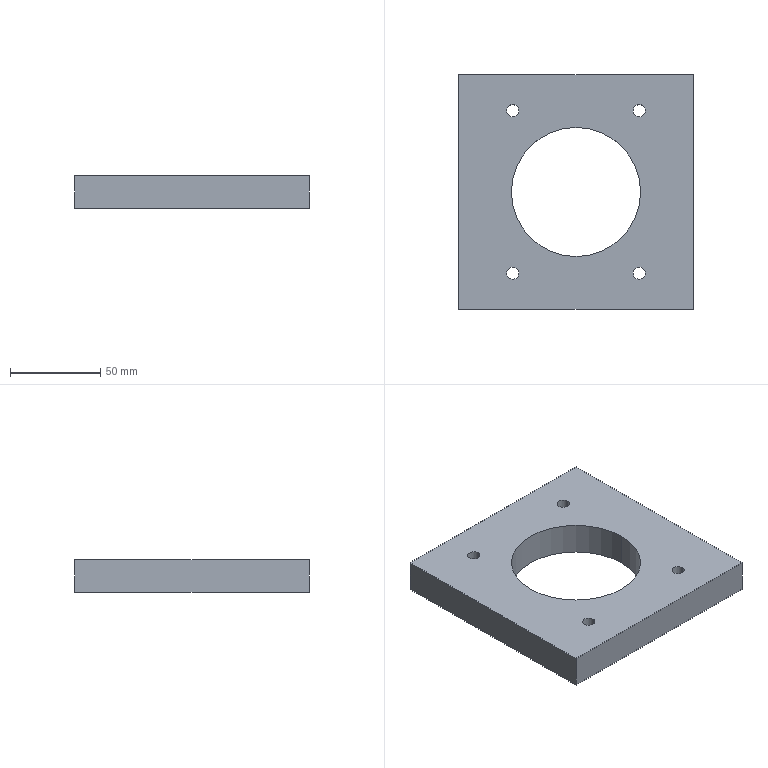Part | SolidWorks | features BaseBody 1 | 1 solid | 24 faces | box 130 x 130 x 18 mm | volume 229251 mm3 | cylinder 10 | cone 8 | plane 6 | commonest cylinder face diameters 6.806 x8 71.52 x2
STEP:
#1=CARTESIAN_POINT('',(-47.597,20.,3.897));
#2=VERTEX_POINT('',#1);
#3=CARTESIAN_POINT('',(-54.403,20.,3.897));
#4=VERTEX_POINT('',#3);
#5=CARTESIAN_POINT('',(-51.,20.,3.897));
#6=DIRECTION('',(0.,0.,-1.));
#7=DIRECTION('',(-1.,0.,0.));
#8=AXIS2_PLACEMENT_3D('',#5,#6,#7);
#9=CIRCLE('',#8,3.403);
#10=EDGE_CURVE('',#2,#4,#9,.T.);
#11=ORIENTED_EDGE('',*,*,#10,.F.);
#12=CARTESIAN_POINT('',(-47.,20.,3.3));
#13=VERTEX_POINT('',#12);
#14=CARTESIAN_POINT('',(-47.,20.,3.3));
#15=DIRECTION('',(0.7071,0.,-0.7071));
#16=VECTOR('',#15,1000.);
#17=LINE('',#14,#16);
#18=EDGE_CURVE('',#2,#13,#17,.T.);
#19=ORIENTED_EDGE('',*,*,#18,.T.);
#20=CARTESIAN_POINT('',(-55.,20.,3.3));
#21=VERTEX_POINT('',#20);
#22=CARTESIAN_POINT('',(-51.,20.,3.3));
#23=DIRECTION('',(0.,0.,-1.));
#24=DIRECTION('',(1.,0.,0.));
#25=AXIS2_PLACEMENT_3D('',#22,#23,#24);
#26=CIRCLE('',#25,4.);
#27=EDGE_CURVE('',#13,#21,#26,.T.);
#28=ORIENTED_EDGE('',*,*,#27,.T.);
#29=CARTESIAN_POINT('',(-55.,20.,3.3));
#30=DIRECTION('',(-0.7071,0.,-0.7071));
#31=VECTOR('',#30,1000.);
#32=LINE('',#29,#31);
#33=EDGE_CURVE('',#4,#21,#32,.T.);
#34=ORIENTED_EDGE('',*,*,#33,.F.);
#35=EDGE_LOOP('',(#11,#19,#28,#34));
#36=FACE_OUTER_BOUND('',#35,.T.);
#37=CARTESIAN_POINT('',(-51.,20.,3.3));
#38=DIRECTION('',(0.,0.,-1.));
#39=DIRECTION('',(-1.,0.,0.));
#40=AXIS2_PLACEMENT_3D('',#37,#38,#39);
#41=CONICAL_SURFACE('',#40,4.,0.7854);
#42=ADVANCED_FACE('',(#36),#41,.F.);
#43=ORIENTED_EDGE('',*,*,#10,.T.);
#44=CARTESIAN_POINT('',(-54.403,20.,21.3));
#45=VERTEX_POINT('',#44);
#46=CARTESIAN_POINT('',(-54.403,20.,-28.7));
#47=DIRECTION('',(0.,0.,1.));
#48=VECTOR('',#47,1000.);
#49=LINE('',#46,#48);
#50=EDGE_CURVE('',#4,#45,#49,.T.);
#51=ORIENTED_EDGE('',*,*,#50,.T.);
#52=CARTESIAN_POINT('',(-47.597,20.,21.3));
#53=VERTEX_POINT('',#52);
#54=CARTESIAN_POINT('',(-51.,20.,21.3));
#55=DIRECTION('',(0.,0.,-1.));
#56=DIRECTION('',(-1.,0.,0.));
#57=AXIS2_PLACEMENT_3D('',#54,#55,#56);
#58=CIRCLE('',#57,3.403);
#59=EDGE_CURVE('',#53,#45,#58,.T.);
#60=ORIENTED_EDGE('',*,*,#59,.F.);
#61=CARTESIAN_POINT('',(-47.597,20.,-28.7));
#62=DIRECTION('',(0.,0.,1.));
#63=VECTOR('',#62,1000.);
#64=LINE('',#61,#63);
#65=EDGE_CURVE('',#2,#53,#64,.T.);
#66=ORIENTED_EDGE('',*,*,#65,.F.);
#67=EDGE_LOOP('',(#43,#51,#60,#66));
#68=FACE_OUTER_BOUND('',#67,.T.);
#69=CARTESIAN_POINT('',(-51.,20.,-28.7));
#70=DIRECTION('',(0.,0.,1.));
#71=DIRECTION('',(1.,0.,0.));
#72=AXIS2_PLACEMENT_3D('',#69,#70,#71);
#73=CYLINDRICAL_SURFACE('',#72,3.403);
#74=ADVANCED_FACE('',(#68),#73,.F.);
#75=CARTESIAN_POINT('',(-117.597,20.,3.897));
#76=VERTEX_POINT('',#75);
#77=CARTESIAN_POINT('',(-124.403,20.,3.897));
#78=VERTEX_POINT('',#77);
#79=CARTESIAN_POINT('',(-121.,20.,3.897));
#80=DIRECTION('',(0.,0.,-1.));
#81=DIRECTION('',(-1.,0.,0.));
#82=AXIS2_PLACEMENT_3D('',#79,#80,#81);
#83=CIRCLE('',#82,3.403);
#84=EDGE_CURVE('',#76,#78,#83,.T.);
#85=ORIENTED_EDGE('',*,*,#84,.F.);
#86=CARTESIAN_POINT('',(-117.,20.,3.3));
#87=VERTEX_POINT('',#86);
#88=CARTESIAN_POINT('',(-117.,20.,3.3));
#89=DIRECTION('',(0.7071,0.,-0.7071));
#90=VECTOR('',#89,1000.);
#91=LINE('',#88,#90);
#92=EDGE_CURVE('',#76,#87,#91,.T.);
#93=ORIENTED_EDGE('',*,*,#92,.T.);
#94=CARTESIAN_POINT('',(-125.,20.,3.3));
#95=VERTEX_POINT('',#94);
#96=CARTESIAN_POINT('',(-121.,20.,3.3));
#97=DIRECTION('',(0.,0.,-1.));
#98=DIRECTION('',(1.,0.,0.));
#99=AXIS2_PLACEMENT_3D('',#96,#97,#98);
#100=CIRCLE('',#99,4.);
#101=EDGE_CURVE('',#87,#95,#100,.T.);
#102=ORIENTED_EDGE('',*,*,#101,.T.);
#103=CARTESIAN_POINT('',(-125.,20.,3.3));
#104=DIRECTION('',(-0.7071,0.,-0.7071));
#105=VECTOR('',#104,1000.);
#106=LINE('',#103,#105);
#107=EDGE_CURVE('',#78,#95,#106,.T.);
#108=ORIENTED_EDGE('',*,*,#107,.F.);
#109=EDGE_LOOP('',(#85,#93,#102,#108));
#110=FACE_OUTER_BOUND('',#109,.T.);
#111=CARTESIAN_POINT('',(-121.,20.,3.3));
#112=DIRECTION('',(0.,0.,-1.));
#113=DIRECTION('',(-1.,0.,0.));
#114=AXIS2_PLACEMENT_3D('',#111,#112,#113);
#115=CONICAL_SURFACE('',#114,4.,0.7854);
#116=ADVANCED_FACE('',(#110),#115,.F.);
#117=ORIENTED_EDGE('',*,*,#84,.T.);
#118=CARTESIAN_POINT('',(-124.403,20.,21.3));
#119=VERTEX_POINT('',#118);
#120=CARTESIAN_POINT('',(-124.403,20.,-28.7));
#121=DIRECTION('',(0.,0.,1.));
#122=VECTOR('',#121,1000.);
#123=LINE('',#120,#122);
#124=EDGE_CURVE('',#78,#119,#123,.T.);
#125=ORIENTED_EDGE('',*,*,#124,.T.);
#126=CARTESIAN_POINT('',(-117.597,20.,21.3));
#127=VERTEX_POINT('',#126);
#128=CARTESIAN_POINT('',(-121.,20.,21.3));
#129=DIRECTION('',(0.,0.,-1.));
#130=DIRECTION('',(-1.,0.,0.));
#131=AXIS2_PLACEMENT_3D('',#128,#129,#130);
#132=CIRCLE('',#131,3.403);
#133=EDGE_CURVE('',#127,#119,#132,.T.);
#134=ORIENTED_EDGE('',*,*,#133,.F.);
#135=CARTESIAN_POINT('',(-117.597,20.,-28.7));
#136=DIRECTION('',(0.,0.,1.));
#137=VECTOR('',#136,1000.);
#138=LINE('',#135,#137);
#139=EDGE_CURVE('',#76,#127,#138,.T.);
#140=ORIENTED_EDGE('',*,*,#139,.F.);
#141=EDGE_LOOP('',(#117,#125,#134,#140));
#142=FACE_OUTER_BOUND('',#141,.T.);
#143=CARTESIAN_POINT('',(-121.,20.,-28.7));
#144=DIRECTION('',(0.,0.,1.));
#145=DIRECTION('',(1.,0.,0.));
#146=AXIS2_PLACEMENT_3D('',#143,#144,#145);
#147=CYLINDRICAL_SURFACE('',#146,3.403);
#148=ADVANCED_FACE('',(#142),#147,.F.);
#149=CARTESIAN_POINT('',(-117.597,-70.,3.897));
#150=VERTEX_POINT('',#149);
#151=CARTESIAN_POINT('',(-124.403,-70.,3.897));
#152=VERTEX_POINT('',#151);
#153=CARTESIAN_POINT('',(-121.,-70.,3.897));
#154=DIRECTION('',(0.,0.,-1.));
#155=DIRECTION('',(-1.,0.,0.));
#156=AXIS2_PLACEMENT_3D('',#153,#154,#155);
#157=CIRCLE('',#156,3.403);
#158=EDGE_CURVE('',#150,#152,#157,.T.);
#159=ORIENTED_EDGE('',*,*,#158,.F.);
#160=CARTESIAN_POINT('',(-117.,-70.,3.3));
#161=VERTEX_POINT('',#160);
#162=CARTESIAN_POINT('',(-117.,-70.,3.3));
#163=DIRECTION('',(0.7071,0.,-0.7071));
#164=VECTOR('',#163,1000.);
#165=LINE('',#162,#164);
#166=EDGE_CURVE('',#150,#161,#165,.T.);
#167=ORIENTED_EDGE('',*,*,#166,.T.);
#168=CARTESIAN_POINT('',(-125.,-70.,3.3));
#169=VERTEX_POINT('',#168);
#170=CARTESIAN_POINT('',(-121.,-70.,3.3));
#171=DIRECTION('',(0.,0.,-1.));
#172=DIRECTION('',(1.,0.,0.));
#173=AXIS2_PLACEMENT_3D('',#170,#171,#172);
#174=CIRCLE('',#173,4.);
#175=EDGE_CURVE('',#161,#169,#174,.T.);
#176=ORIENTED_EDGE('',*,*,#175,.T.);
#177=CARTESIAN_POINT('',(-125.,-70.,3.3));
#178=DIRECTION('',(-0.7071,0.,-0.7071));
#179=VECTOR('',#178,1000.);
#180=LINE('',#177,#179);
#181=EDGE_CURVE('',#152,#169,#180,.T.);
#182=ORIENTED_EDGE('',*,*,#181,.F.);
#183=EDGE_LOOP('',(#159,#167,#176,#182));
#184=FACE_OUTER_BOUND('',#183,.T.);
#185=CARTESIAN_POINT('',(-121.,-70.,3.3));
#186=DIRECTION('',(0.,0.,-1.));
#187=DIRECTION('',(-1.,0.,0.));
#188=AXIS2_PLACEMENT_3D('',#185,#186,#187);
#189=CONICAL_SURFACE('',#188,4.,0.7854);
#190=ADVANCED_FACE('',(#184),#189,.F.);
#191=ORIENTED_EDGE('',*,*,#158,.T.);
#192=CARTESIAN_POINT('',(-124.403,-70.,21.3));
#193=VERTEX_POINT('',#192);
#194=CARTESIAN_POINT('',(-124.403,-70.,-28.7));
#195=DIRECTION('',(0.,0.,1.));
#196=VECTOR('',#195,1000.);
#197=LINE('',#194,#196);
#198=EDGE_CURVE('',#152,#193,#197,.T.);
#199=ORIENTED_EDGE('',*,*,#198,.T.);
#200=CARTESIAN_POINT('',(-117.597,-70.,21.3));
#201=VERTEX_POINT('',#200);
#202=CARTESIAN_POINT('',(-121.,-70.,21.3));
#203=DIRECTION('',(0.,0.,-1.));
#204=DIRECTION('',(-1.,0.,0.));
#205=AXIS2_PLACEMENT_3D('',#202,#203,#204);
#206=CIRCLE('',#205,3.403);
#207=EDGE_CURVE('',#201,#193,#206,.T.);
#208=ORIENTED_EDGE('',*,*,#207,.F.);
#209=CARTESIAN_POINT('',(-117.597,-70.,-28.7));
#210=DIRECTION('',(0.,0.,1.));
#211=VECTOR('',#210,1000.);
#212=LINE('',#209,#211);
#213=EDGE_CURVE('',#150,#201,#212,.T.);
#214=ORIENTED_EDGE('',*,*,#213,.F.);
#215=EDGE_LOOP('',(#191,#199,#208,#214));
#216=FACE_OUTER_BOUND('',#215,.T.);
#217=CARTESIAN_POINT('',(-121.,-70.,-28.7));
#218=DIRECTION('',(0.,0.,1.));
#219=DIRECTION('',(1.,0.,0.));
#220=AXIS2_PLACEMENT_3D('',#217,#218,#219);
#221=CYLINDRICAL_SURFACE('',#220,3.403);
#222=ADVANCED_FACE('',(#216),#221,.F.);
#223=CARTESIAN_POINT('',(-47.597,-70.,3.897));
#224=VERTEX_POINT('',#223);
#225=CARTESIAN_POINT('',(-54.403,-70.,3.897));
#226=VERTEX_POINT('',#225);
#227=CARTESIAN_POINT('',(-51.,-70.,3.897));
#228=DIRECTION('',(0.,0.,-1.));
#229=DIRECTION('',(-1.,0.,0.));
#230=AXIS2_PLACEMENT_3D('',#227,#228,#229);
#231=CIRCLE('',#230,3.403);
#232=EDGE_CURVE('',#224,#226,#231,.T.);
#233=ORIENTED_EDGE('',*,*,#232,.F.);
#234=CARTESIAN_POINT('',(-47.,-70.,3.3));
#235=VERTEX_POINT('',#234);
#236=CARTESIAN_POINT('',(-47.,-70.,3.3));
#237=DIRECTION('',(0.7071,0.,-0.7071));
#238=VECTOR('',#237,1000.);
#239=LINE('',#236,#238);
#240=EDGE_CURVE('',#224,#235,#239,.T.);
#241=ORIENTED_EDGE('',*,*,#240,.T.);
#242=CARTESIAN_POINT('',(-55.,-70.,3.3));
#243=VERTEX_POINT('',#242);
#244=CARTESIAN_POINT('',(-51.,-70.,3.3));
#245=DIRECTION('',(0.,0.,-1.));
#246=DIRECTION('',(1.,0.,0.));
#247=AXIS2_PLACEMENT_3D('',#244,#245,#246);
#248=CIRCLE('',#247,4.);
#249=EDGE_CURVE('',#235,#243,#248,.T.);
#250=ORIENTED_EDGE('',*,*,#249,.T.);
#251=CARTESIAN_POINT('',(-55.,-70.,3.3));
#252=DIRECTION('',(-0.7071,0.,-0.7071));
#253=VECTOR('',#252,1000.);
#254=LINE('',#251,#253);
#255=EDGE_CURVE('',#226,#243,#254,.T.);
#256=ORIENTED_EDGE('',*,*,#255,.F.);
#257=EDGE_LOOP('',(#233,#241,#250,#256));
#258=FACE_OUTER_BOUND('',#257,.T.);
#259=CARTESIAN_POINT('',(-51.,-70.,3.3));
#260=DIRECTION('',(0.,0.,-1.));
#261=DIRECTION('',(-1.,0.,0.));
#262=AXIS2_PLACEMENT_3D('',#259,#260,#261);
#263=CONICAL_SURFACE('',#262,4.,0.7854);
#264=ADVANCED_FACE('',(#258),#263,.F.);
#265=ORIENTED_EDGE('',*,*,#232,.T.);
#266=CARTESIAN_POINT('',(-54.403,-70.,21.3));
#267=VERTEX_POINT('',#266);
#268=CARTESIAN_POINT('',(-54.403,-70.,-28.7));
#269=DIRECTION('',(0.,0.,1.));
#270=VECTOR('',#269,1000.);
#271=LINE('',#268,#270);
#272=EDGE_CURVE('',#226,#267,#271,.T.);
#273=ORIENTED_EDGE('',*,*,#272,.T.);
#274=CARTESIAN_POINT('',(-47.597,-70.,21.3));
#275=VERTEX_POINT('',#274);
#276=CARTESIAN_POINT('',(-51.,-70.,21.3));
#277=DIRECTION('',(0.,0.,-1.));
#278=DIRECTION('',(-1.,0.,0.));
#279=AXIS2_PLACEMENT_3D('',#276,#277,#278);
#280=CIRCLE('',#279,3.403);
#281=EDGE_CURVE('',#275,#267,#280,.T.);
#282=ORIENTED_EDGE('',*,*,#281,.F.);
#283=CARTESIAN_POINT('',(-47.597,-70.,-28.7));
#284=DIRECTION('',(0.,0.,1.));
#285=VECTOR('',#284,1000.);
#286=LINE('',#283,#285);
#287=EDGE_CURVE('',#224,#275,#286,.T.);
#288=ORIENTED_EDGE('',*,*,#287,.F.);
#289=EDGE_LOOP('',(#265,#273,#282,#288));
#290=FACE_OUTER_BOUND('',#289,.T.);
#291=CARTESIAN_POINT('',(-51.,-70.,-28.7));
#292=DIRECTION('',(0.,0.,1.));
#293=DIRECTION('',(1.,0.,0.));
#294=AXIS2_PLACEMENT_3D('',#291,#292,#293);
#295=CYLINDRICAL_SURFACE('',#294,3.403);
#296=ADVANCED_FACE('',(#290),#295,.F.);
#297=CARTESIAN_POINT('',(-50.24,-25.,21.3));
#298=VERTEX_POINT('',#297);
#299=CARTESIAN_POINT('',(-121.76,-25.,21.3));
#300=VERTEX_POINT('',#299);
#301=CARTESIAN_POINT('',(-86.,-25.,21.3));
#302=DIRECTION('',(0.,0.,-1.));
#303=DIRECTION('',(-1.,0.,0.));
#304=AXIS2_PLACEMENT_3D('',#301,#302,#303);
#305=CIRCLE('',#304,35.76);
#306=EDGE_CURVE('',#298,#300,#305,.T.);
#307=ORIENTED_EDGE('',*,*,#306,.F.);
#308=CARTESIAN_POINT('',(-50.24,-25.,3.3));
#309=VERTEX_POINT('',#308);
#310=CARTESIAN_POINT('',(-50.24,-25.,141.4));
#311=DIRECTION('',(0.,0.,-1.));
#312=VECTOR('',#311,1000.);
#313=LINE('',#310,#312);
#314=EDGE_CURVE('',#298,#309,#313,.T.);
#315=ORIENTED_EDGE('',*,*,#314,.T.);
#316=CARTESIAN_POINT('',(-121.76,-25.,3.3));
#317=VERTEX_POINT('',#316);
#318=CARTESIAN_POINT('',(-86.,-25.,3.3));
#319=DIRECTION('',(0.,0.,-1.));
#320=DIRECTION('',(-1.,0.,0.));
#321=AXIS2_PLACEMENT_3D('',#318,#319,#320);
#322=CIRCLE('',#321,35.76);
#323=EDGE_CURVE('',#309,#317,#322,.T.);
#324=ORIENTED_EDGE('',*,*,#323,.T.);
#325=CARTESIAN_POINT('',(-121.76,-25.,141.4));
#326=DIRECTION('',(0.,0.,-1.));
#327=VECTOR('',#326,1000.);
#328=LINE('',#325,#327);
#329=EDGE_CURVE('',#300,#317,#328,.T.);
#330=ORIENTED_EDGE('',*,*,#329,.F.);
#331=EDGE_LOOP('',(#307,#315,#324,#330));
#332=FACE_OUTER_BOUND('',#331,.T.);
#333=CARTESIAN_POINT('',(-86.,-25.,141.4));
#334=DIRECTION('',(0.,0.,-1.));
#335=DIRECTION('',(-1.,0.,0.));
#336=AXIS2_PLACEMENT_3D('',#333,#334,#335);
#337=CYLINDRICAL_SURFACE('',#336,35.76);
#338=ADVANCED_FACE('',(#332),#337,.F.);
#339=CARTESIAN_POINT('',(-51.,20.,3.3));
#340=DIRECTION('',(0.,0.,-1.));
#341=DIRECTION('',(1.,0.,0.));
#342=AXIS2_PLACEMENT_3D('',#339,#340,#341);
#343=CIRCLE('',#342,4.);
#344=EDGE_CURVE('',#21,#13,#343,.T.);
#345=ORIENTED_EDGE('',*,*,#344,.F.);
#346=ORIENTED_EDGE('',*,*,#27,.F.);
#347=EDGE_LOOP('',(#345,#346));
#348=FACE_BOUND('',#347,.T.);
#349=CARTESIAN_POINT('',(-121.,20.,3.3));
#350=DIRECTION('',(0.,0.,-1.));
#351=DIRECTION('',(1.,0.,0.));
#352=AXIS2_PLACEMENT_3D('',#349,#350,#351);
#353=CIRCLE('',#352,4.);
#354=EDGE_CURVE('',#95,#87,#353,.T.);
#355=ORIENTED_EDGE('',*,*,#354,.F.);
#356=ORIENTED_EDGE('',*,*,#101,.F.);
#357=EDGE_LOOP('',(#355,#356));
#358=FACE_BOUND('',#357,.T.);
#359=CARTESIAN_POINT('',(-121.,-70.,3.3));
#360=DIRECTION('',(0.,0.,-1.));
#361=DIRECTION('',(1.,0.,0.));
#362=AXIS2_PLACEMENT_3D('',#359,#360,#361);
#363=CIRCLE('',#362,4.);
#364=EDGE_CURVE('',#169,#161,#363,.T.);
#365=ORIENTED_EDGE('',*,*,#364,.F.);
#366=ORIENTED_EDGE('',*,*,#175,.F.);
#367=EDGE_LOOP('',(#365,#366));
#368=FACE_BOUND('',#367,.T.);
#369=CARTESIAN_POINT('',(-51.,-70.,3.3));
#370=DIRECTION('',(0.,0.,-1.));
#371=DIRECTION('',(1.,0.,0.));
#372=AXIS2_PLACEMENT_3D('',#369,#370,#371);
#373=CIRCLE('',#372,4.);
#374=EDGE_CURVE('',#243,#235,#373,.T.);
#375=ORIENTED_EDGE('',*,*,#374,.F.);
#376=ORIENTED_EDGE('',*,*,#249,.F.);
#377=EDGE_LOOP('',(#375,#376));
#378=FACE_BOUND('',#377,.T.);
#379=CARTESIAN_POINT('',(-86.,-25.,3.3));
#380=DIRECTION('',(0.,0.,-1.));
#381=DIRECTION('',(-1.,0.,0.));
#382=AXIS2_PLACEMENT_3D('',#379,#380,#381);
#383=CIRCLE('',#382,35.76);
#384=EDGE_CURVE('',#317,#309,#383,.T.);
#385=ORIENTED_EDGE('',*,*,#384,.F.);
#386=ORIENTED_EDGE('',*,*,#323,.F.);
#387=EDGE_LOOP('',(#385,#386));
#388=FACE_BOUND('',#387,.T.);
#389=CARTESIAN_POINT('',(-151.,-90.,3.3));
#390=VERTEX_POINT('',#389);
#391=CARTESIAN_POINT('',(-21.,-90.,3.3));
#392=VERTEX_POINT('',#391);
#393=CARTESIAN_POINT('',(-86.,-90.,3.3));
#394=DIRECTION('',(1.,0.,0.));
#395=VECTOR('',#394,1000.);
#396=LINE('',#393,#395);
#397=EDGE_CURVE('',#390,#392,#396,.T.);
#398=ORIENTED_EDGE('',*,*,#397,.F.);
#399=CARTESIAN_POINT('',(-151.,40.,3.3));
#400=VERTEX_POINT('',#399);
#401=CARTESIAN_POINT('',(-151.,-25.,3.3));
#402=DIRECTION('',(0.,-1.,0.));
#403=VECTOR('',#402,1000.);
#404=LINE('',#401,#403);
#405=EDGE_CURVE('',#400,#390,#404,.T.);
#406=ORIENTED_EDGE('',*,*,#405,.F.);
#407=CARTESIAN_POINT('',(-21.,40.,3.3));
#408=VERTEX_POINT('',#407);
#409=CARTESIAN_POINT('',(-86.,40.,3.3));
#410=DIRECTION('',(-1.,0.,0.));
#411=VECTOR('',#410,1000.);
#412=LINE('',#409,#411);
#413=EDGE_CURVE('',#408,#400,#412,.T.);
#414=ORIENTED_EDGE('',*,*,#413,.F.);
#415=CARTESIAN_POINT('',(-21.,-25.,3.3));
#416=DIRECTION('',(0.,1.,0.));
#417=VECTOR('',#416,1000.);
#418=LINE('',#415,#417);
#419=EDGE_CURVE('',#392,#408,#418,.T.);
#420=ORIENTED_EDGE('',*,*,#419,.F.);
#421=EDGE_LOOP('',(#398,#406,#414,#420));
#422=FACE_OUTER_BOUND('',#421,.T.);
#423=CARTESIAN_POINT('',(-86.,-25.,3.3));
#424=DIRECTION('',(0.,0.,-1.));
#425=DIRECTION('',(-1.,0.,0.));
#426=AXIS2_PLACEMENT_3D('',#423,#424,#425);
#427=PLANE('',#426);
#428=ADVANCED_FACE('',(#348,#358,#368,#378,#388,#422),#427,.T.);
#429=CARTESIAN_POINT('',(-151.,-90.,21.3));
#430=VERTEX_POINT('',#429);
#431=CARTESIAN_POINT('',(-21.,-90.,21.3));
#432=VERTEX_POINT('',#431);
#433=CARTESIAN_POINT('',(-86.,-90.,21.3));
#434=DIRECTION('',(1.,0.,0.));
#435=VECTOR('',#434,1000.);
#436=LINE('',#433,#435);
#437=EDGE_CURVE('',#430,#432,#436,.T.);
#438=ORIENTED_EDGE('',*,*,#437,.F.);
#439=CARTESIAN_POINT('',(-151.,-90.,41.3));
#440=DIRECTION('',(0.,0.,-1.));
#441=VECTOR('',#440,1000.);
#442=LINE('',#439,#441);
#443=EDGE_CURVE('',#430,#390,#442,.T.);
#444=ORIENTED_EDGE('',*,*,#443,.T.);
#445=ORIENTED_EDGE('',*,*,#397,.T.);
#446=CARTESIAN_POINT('',(-21.,-90.,41.3));
#447=DIRECTION('',(0.,0.,-1.));
#448=VECTOR('',#447,1000.);
#449=LINE('',#446,#448);
#450=EDGE_CURVE('',#432,#392,#449,.T.);
#451=ORIENTED_EDGE('',*,*,#450,.F.);
#452=EDGE_LOOP('',(#438,#444,#445,#451));
#453=FACE_OUTER_BOUND('',#452,.T.);
#454=CARTESIAN_POINT('',(-86.,-90.,41.3));
#455=DIRECTION('',(0.,-1.,0.));
#456=DIRECTION('',(0.,0.,1.));
#457=AXIS2_PLACEMENT_3D('',#454,#455,#456);
#458=PLANE('',#457);
#459=ADVANCED_FACE('',(#453),#458,.T.);
#460=CARTESIAN_POINT('',(-21.,40.,21.3));
#461=VERTEX_POINT('',#460);
#462=CARTESIAN_POINT('',(-21.,-25.,21.3));
#463=DIRECTION('',(0.,1.,0.));
#464=VECTOR('',#463,1000.);
#465=LINE('',#462,#464);
#466=EDGE_CURVE('',#432,#461,#465,.T.);
#467=ORIENTED_EDGE('',*,*,#466,.F.);
#468=ORIENTED_EDGE('',*,*,#450,.T.);
#469=ORIENTED_EDGE('',*,*,#419,.T.);
#470=CARTESIAN_POINT('',(-21.,40.,41.3));
#471=DIRECTION('',(0.,0.,-1.));
#472=VECTOR('',#471,1000.);
#473=LINE('',#470,#472);
#474=EDGE_CURVE('',#461,#408,#473,.T.);
#475=ORIENTED_EDGE('',*,*,#474,.F.);
#476=EDGE_LOOP('',(#467,#468,#469,#475));
#477=FACE_OUTER_BOUND('',#476,.T.);
#478=CARTESIAN_POINT('',(-21.,-25.,41.3));
#479=DIRECTION('',(1.,0.,0.));
#480=DIRECTION('',(0.,0.,-1.));
#481=AXIS2_PLACEMENT_3D('',#478,#479,#480);
#482=PLANE('',#481);
#483=ADVANCED_FACE('',(#477),#482,.T.);
#484=CARTESIAN_POINT('',(-151.,40.,21.3));
#485=VERTEX_POINT('',#484);
#486=CARTESIAN_POINT('',(-86.,40.,21.3));
#487=DIRECTION('',(-1.,0.,0.));
#488=VECTOR('',#487,1000.);
#489=LINE('',#486,#488);
#490=EDGE_CURVE('',#461,#485,#489,.T.);
#491=ORIENTED_EDGE('',*,*,#490,.F.);
#492=ORIENTED_EDGE('',*,*,#474,.T.);
#493=ORIENTED_EDGE('',*,*,#413,.T.);
#494=CARTESIAN_POINT('',(-151.,40.,41.3));
#495=DIRECTION('',(0.,0.,-1.));
#496=VECTOR('',#495,1000.);
#497=LINE('',#494,#496);
#498=EDGE_CURVE('',#485,#400,#497,.T.);
#499=ORIENTED_EDGE('',*,*,#498,.F.);
#500=EDGE_LOOP('',(#491,#492,#493,#499));
#501=FACE_OUTER_BOUND('',#500,.T.);
#502=CARTESIAN_POINT('',(-86.,40.,41.3));
#503=DIRECTION('',(0.,1.,0.));
#504=DIRECTION('',(0.,0.,-1.));
#505=AXIS2_PLACEMENT_3D('',#502,#503,#504);
#506=PLANE('',#505);
#507=ADVANCED_FACE('',(#501),#506,.T.);
#508=CARTESIAN_POINT('',(-151.,-25.,21.3));
#509=DIRECTION('',(0.,-1.,0.));
#510=VECTOR('',#509,1000.);
#511=LINE('',#508,#510);
#512=EDGE_CURVE('',#485,#430,#511,.T.);
#513=ORIENTED_EDGE('',*,*,#512,.F.);
#514=ORIENTED_EDGE('',*,*,#498,.T.);
#515=ORIENTED_EDGE('',*,*,#405,.T.);
#516=ORIENTED_EDGE('',*,*,#443,.F.);
#517=EDGE_LOOP('',(#513,#514,#515,#516));
#518=FACE_OUTER_BOUND('',#517,.T.);
#519=CARTESIAN_POINT('',(-151.,-25.,41.3));
#520=DIRECTION('',(-1.,0.,0.));
#521=DIRECTION('',(0.,0.,1.));
#522=AXIS2_PLACEMENT_3D('',#519,#520,#521);
#523=PLANE('',#522);
#524=ADVANCED_FACE('',(#518),#523,.T.);
#525=ORIENTED_EDGE('',*,*,#59,.T.);
#526=CARTESIAN_POINT('',(-51.,20.,21.3));
#527=DIRECTION('',(0.,0.,-1.));
#528=DIRECTION('',(-1.,0.,0.));
#529=AXIS2_PLACEMENT_3D('',#526,#527,#528);
#530=CIRCLE('',#529,3.403);
#531=EDGE_CURVE('',#45,#53,#530,.T.);
#532=ORIENTED_EDGE('',*,*,#531,.T.);
#533=EDGE_LOOP('',(#525,#532));
#534=FACE_BOUND('',#533,.T.);
#535=ORIENTED_EDGE('',*,*,#133,.T.);
#536=CARTESIAN_POINT('',(-121.,20.,21.3));
#537=DIRECTION('',(0.,0.,-1.));
#538=DIRECTION('',(-1.,0.,0.));
#539=AXIS2_PLACEMENT_3D('',#536,#537,#538);
#540=CIRCLE('',#539,3.403);
#541=EDGE_CURVE('',#119,#127,#540,.T.);
#542=ORIENTED_EDGE('',*,*,#541,.T.);
#543=EDGE_LOOP('',(#535,#542));
#544=FACE_BOUND('',#543,.T.);
#545=ORIENTED_EDGE('',*,*,#207,.T.);
#546=CARTESIAN_POINT('',(-121.,-70.,21.3));
#547=DIRECTION('',(0.,0.,-1.));
#548=DIRECTION('',(-1.,0.,0.));
#549=AXIS2_PLACEMENT_3D('',#546,#547,#548);
#550=CIRCLE('',#549,3.403);
#551=EDGE_CURVE('',#193,#201,#550,.T.);
#552=ORIENTED_EDGE('',*,*,#551,.T.);
#553=EDGE_LOOP('',(#545,#552));
#554=FACE_BOUND('',#553,.T.);
#555=ORIENTED_EDGE('',*,*,#281,.T.);
#556=CARTESIAN_POINT('',(-51.,-70.,21.3));
#557=DIRECTION('',(0.,0.,-1.));
#558=DIRECTION('',(-1.,0.,0.));
#559=AXIS2_PLACEMENT_3D('',#556,#557,#558);
#560=CIRCLE('',#559,3.403);
#561=EDGE_CURVE('',#267,#275,#560,.T.);
#562=ORIENTED_EDGE('',*,*,#561,.T.);
#563=EDGE_LOOP('',(#555,#562));
#564=FACE_BOUND('',#563,.T.);
#565=CARTESIAN_POINT('',(-86.,-25.,21.3));
#566=DIRECTION('',(0.,0.,-1.));
#567=DIRECTION('',(-1.,0.,0.));
#568=AXIS2_PLACEMENT_3D('',#565,#566,#567);
#569=CIRCLE('',#568,35.76);
#570=EDGE_CURVE('',#300,#298,#569,.T.);
#571=ORIENTED_EDGE('',*,*,#570,.T.);
#572=ORIENTED_EDGE('',*,*,#306,.T.);
#573=EDGE_LOOP('',(#571,#572));
#574=FACE_BOUND('',#573,.T.);
#575=ORIENTED_EDGE('',*,*,#437,.T.);
#576=ORIENTED_EDGE('',*,*,#466,.T.);
#577=ORIENTED_EDGE('',*,*,#490,.T.);
#578=ORIENTED_EDGE('',*,*,#512,.T.);
#579=EDGE_LOOP('',(#575,#576,#577,#578));
#580=FACE_OUTER_BOUND('',#579,.T.);
#581=CARTESIAN_POINT('',(-86.,-25.,21.3));
#582=DIRECTION('',(0.,0.,-1.));
#583=DIRECTION('',(-1.,0.,0.));
#584=AXIS2_PLACEMENT_3D('',#581,#582,#583);
#585=PLANE('',#584);
#586=ADVANCED_FACE('',(#534,#544,#554,#564,#574,#580),#585,.F.);
#587=ORIENTED_EDGE('',*,*,#314,.F.);
#588=ORIENTED_EDGE('',*,*,#570,.F.);
#589=ORIENTED_EDGE('',*,*,#329,.T.);
#590=ORIENTED_EDGE('',*,*,#384,.T.);
#591=EDGE_LOOP('',(#587,#588,#589,#590));
#592=FACE_OUTER_BOUND('',#591,.T.);
#593=CARTESIAN_POINT('',(-86.,-25.,141.4));
#594=DIRECTION('',(0.,0.,-1.));
#595=DIRECTION('',(-1.,0.,0.));
#596=AXIS2_PLACEMENT_3D('',#593,#594,#595);
#597=CYLINDRICAL_SURFACE('',#596,35.76);
#598=ADVANCED_FACE('',(#592),#597,.F.);
#599=ORIENTED_EDGE('',*,*,#272,.F.);
#600=CARTESIAN_POINT('',(-51.,-70.,3.897));
#601=DIRECTION('',(0.,0.,-1.));
#602=DIRECTION('',(-1.,0.,0.));
#603=AXIS2_PLACEMENT_3D('',#600,#601,#602);
#604=CIRCLE('',#603,3.403);
#605=EDGE_CURVE('',#226,#224,#604,.T.);
#606=ORIENTED_EDGE('',*,*,#605,.T.);
#607=ORIENTED_EDGE('',*,*,#287,.T.);
#608=ORIENTED_EDGE('',*,*,#561,.F.);
#609=EDGE_LOOP('',(#599,#606,#607,#608));
#610=FACE_OUTER_BOUND('',#609,.T.);
#611=CARTESIAN_POINT('',(-51.,-70.,-28.7));
#612=DIRECTION('',(0.,0.,1.));
#613=DIRECTION('',(1.,0.,0.));
#614=AXIS2_PLACEMENT_3D('',#611,#612,#613);
#615=CYLINDRICAL_SURFACE('',#614,3.403);
#616=ADVANCED_FACE('',(#610),#615,.F.);
#617=ORIENTED_EDGE('',*,*,#240,.F.);
#618=ORIENTED_EDGE('',*,*,#605,.F.);
#619=ORIENTED_EDGE('',*,*,#255,.T.);
#620=ORIENTED_EDGE('',*,*,#374,.T.);
#621=EDGE_LOOP('',(#617,#618,#619,#620));
#622=FACE_OUTER_BOUND('',#621,.T.);
#623=CARTESIAN_POINT('',(-51.,-70.,3.3));
#624=DIRECTION('',(0.,0.,-1.));
#625=DIRECTION('',(-1.,0.,0.));
#626=AXIS2_PLACEMENT_3D('',#623,#624,#625);
#627=CONICAL_SURFACE('',#626,4.,0.7854);
#628=ADVANCED_FACE('',(#622),#627,.F.);
#629=ORIENTED_EDGE('',*,*,#198,.F.);
#630=CARTESIAN_POINT('',(-121.,-70.,3.897));
#631=DIRECTION('',(0.,0.,-1.));
#632=DIRECTION('',(-1.,0.,0.));
#633=AXIS2_PLACEMENT_3D('',#630,#631,#632);
#634=CIRCLE('',#633,3.403);
#635=EDGE_CURVE('',#152,#150,#634,.T.);
#636=ORIENTED_EDGE('',*,*,#635,.T.);
#637=ORIENTED_EDGE('',*,*,#213,.T.);
#638=ORIENTED_EDGE('',*,*,#551,.F.);
#639=EDGE_LOOP('',(#629,#636,#637,#638));
#640=FACE_OUTER_BOUND('',#639,.T.);
#641=CARTESIAN_POINT('',(-121.,-70.,-28.7));
#642=DIRECTION('',(0.,0.,1.));
#643=DIRECTION('',(1.,0.,0.));
#644=AXIS2_PLACEMENT_3D('',#641,#642,#643);
#645=CYLINDRICAL_SURFACE('',#644,3.403);
#646=ADVANCED_FACE('',(#640),#645,.F.);
#647=ORIENTED_EDGE('',*,*,#166,.F.);
#648=ORIENTED_EDGE('',*,*,#635,.F.);
#649=ORIENTED_EDGE('',*,*,#181,.T.);
#650=ORIENTED_EDGE('',*,*,#364,.T.);
#651=EDGE_LOOP('',(#647,#648,#649,#650));
#652=FACE_OUTER_BOUND('',#651,.T.);
#653=CARTESIAN_POINT('',(-121.,-70.,3.3));
#654=DIRECTION('',(0.,0.,-1.));
#655=DIRECTION('',(-1.,0.,0.));
#656=AXIS2_PLACEMENT_3D('',#653,#654,#655);
#657=CONICAL_SURFACE('',#656,4.,0.7854);
#658=ADVANCED_FACE('',(#652),#657,.F.);
#659=ORIENTED_EDGE('',*,*,#124,.F.);
#660=CARTESIAN_POINT('',(-121.,20.,3.897));
#661=DIRECTION('',(0.,0.,-1.));
#662=DIRECTION('',(-1.,0.,0.));
#663=AXIS2_PLACEMENT_3D('',#660,#661,#662);
#664=CIRCLE('',#663,3.403);
#665=EDGE_CURVE('',#78,#76,#664,.T.);
#666=ORIENTED_EDGE('',*,*,#665,.T.);
#667=ORIENTED_EDGE('',*,*,#139,.T.);
#668=ORIENTED_EDGE('',*,*,#541,.F.);
#669=EDGE_LOOP('',(#659,#666,#667,#668));
#670=FACE_OUTER_BOUND('',#669,.T.);
#671=CARTESIAN_POINT('',(-121.,20.,-28.7));
#672=DIRECTION('',(0.,0.,1.));
#673=DIRECTION('',(1.,0.,0.));
#674=AXIS2_PLACEMENT_3D('',#671,#672,#673);
#675=CYLINDRICAL_SURFACE('',#674,3.403);
#676=ADVANCED_FACE('',(#670),#675,.F.);
#677=ORIENTED_EDGE('',*,*,#92,.F.);
#678=ORIENTED_EDGE('',*,*,#665,.F.);
#679=ORIENTED_EDGE('',*,*,#107,.T.);
#680=ORIENTED_EDGE('',*,*,#354,.T.);
#681=EDGE_LOOP('',(#677,#678,#679,#680));
#682=FACE_OUTER_BOUND('',#681,.T.);
#683=CARTESIAN_POINT('',(-121.,20.,3.3));
#684=DIRECTION('',(0.,0.,-1.));
#685=DIRECTION('',(-1.,0.,0.));
#686=AXIS2_PLACEMENT_3D('',#683,#684,#685);
#687=CONICAL_SURFACE('',#686,4.,0.7854);
#688=ADVANCED_FACE('',(#682),#687,.F.);
#689=ORIENTED_EDGE('',*,*,#50,.F.);
#690=CARTESIAN_POINT('',(-51.,20.,3.897));
#691=DIRECTION('',(0.,0.,-1.));
#692=DIRECTION('',(-1.,0.,0.));
#693=AXIS2_PLACEMENT_3D('',#690,#691,#692);
#694=CIRCLE('',#693,3.403);
#695=EDGE_CURVE('',#4,#2,#694,.T.);
#696=ORIENTED_EDGE('',*,*,#695,.T.);
#697=ORIENTED_EDGE('',*,*,#65,.T.);
#698=ORIENTED_EDGE('',*,*,#531,.F.);
#699=EDGE_LOOP('',(#689,#696,#697,#698));
#700=FACE_OUTER_BOUND('',#699,.T.);
#701=CARTESIAN_POINT('',(-51.,20.,-28.7));
#702=DIRECTION('',(0.,0.,1.));
#703=DIRECTION('',(1.,0.,0.));
#704=AXIS2_PLACEMENT_3D('',#701,#702,#703);
#705=CYLINDRICAL_SURFACE('',#704,3.403);
#706=ADVANCED_FACE('',(#700),#705,.F.);
#707=ORIENTED_EDGE('',*,*,#18,.F.);
#708=ORIENTED_EDGE('',*,*,#695,.F.);
#709=ORIENTED_EDGE('',*,*,#33,.T.);
#710=ORIENTED_EDGE('',*,*,#344,.T.);
#711=EDGE_LOOP('',(#707,#708,#709,#710));
#712=FACE_OUTER_BOUND('',#711,.T.);
#713=CARTESIAN_POINT('',(-51.,20.,3.3));
#714=DIRECTION('',(0.,0.,-1.));
#715=DIRECTION('',(-1.,0.,0.));
#716=AXIS2_PLACEMENT_3D('',#713,#714,#715);
#717=CONICAL_SURFACE('',#716,4.,0.7854);
#718=ADVANCED_FACE('',(#712),#717,.F.);
#719=CLOSED_SHELL('',(#42,#74,#116,#148,#190,#222,#264,#296,#338,#428,#459,#483,#507,#524,#586,#598,#616,#628,#646,#658,#676,#688,#706,#718));
#720=MANIFOLD_SOLID_BREP('',#719);
#721=CARTESIAN_POINT('',(0.,0.,0.));
#722=DIRECTION('',(0.,0.,1.));
#723=DIRECTION('',(1.,0.,0.));
#724=AXIS2_PLACEMENT_3D('',#721,#722,#723);
#725=(LENGTH_UNIT()NAMED_UNIT(*)SI_UNIT(.MILLI.,.METRE.));
#726=UNCERTAINTY_MEASURE_WITH_UNIT(LENGTH_MEASURE(0.00001),#725,'','');
#727=(NAMED_UNIT(*)PLANE_ANGLE_UNIT()SI_UNIT($,.RADIAN.));
#728=(NAMED_UNIT(*)SI_UNIT($,.STERADIAN.)SOLID_ANGLE_UNIT());
#729=(GEOMETRIC_REPRESENTATION_CONTEXT(3)GLOBAL_UNCERTAINTY_ASSIGNED_CONTEXT((#726))GLOBAL_UNIT_ASSIGNED_CONTEXT((#725,#727,#728))REPRESENTATION_CONTEXT('',''));
#730=ADVANCED_BREP_SHAPE_REPRESENTATION('',(#720,#724),#729);